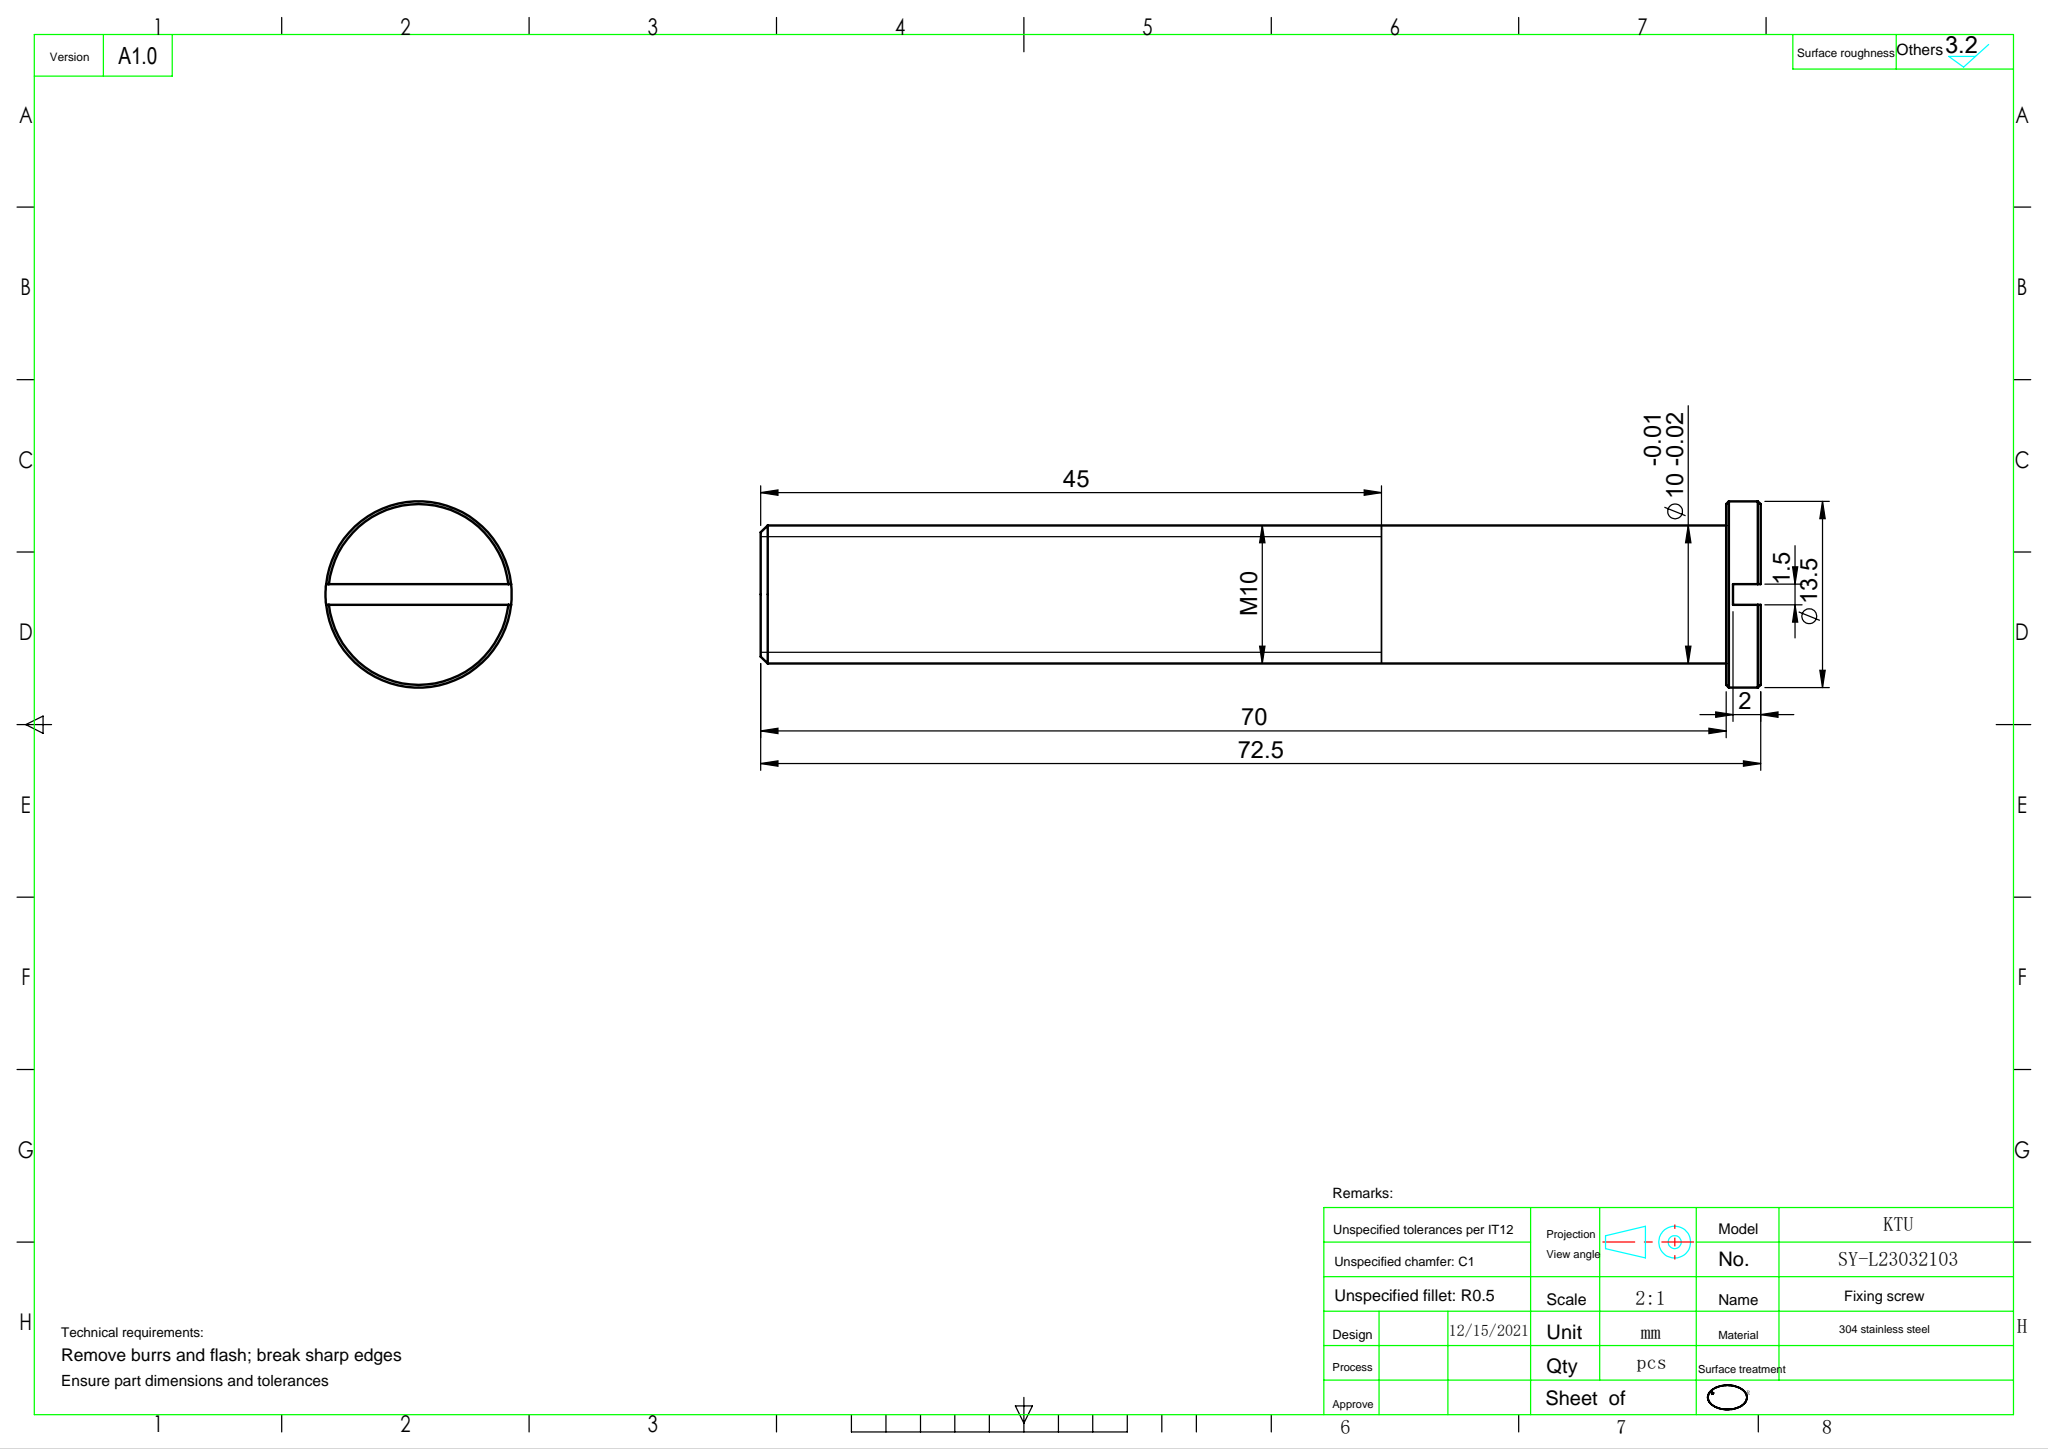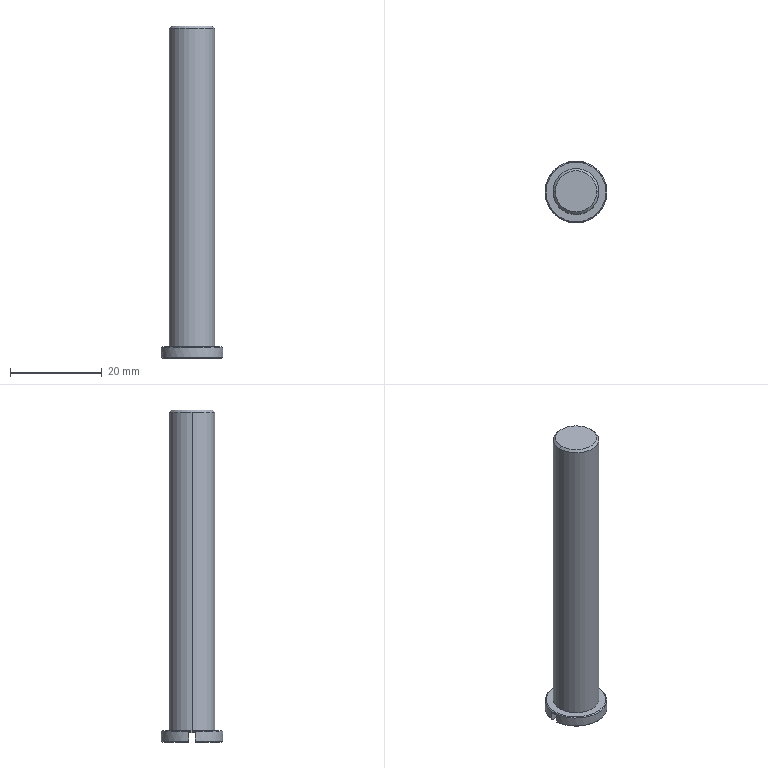Part | SolidWorks | features Chamfer 2, ICE 2, Extrusion 1 | 1 solid | 17 faces | box 13.5 x 13.5 x 72.5 mm | volume 5810 mm3 | plane 7 | cone 6 | cylinder 4 | commonest cylinder face diameters 10 x2 13.5 x2
STEP:
#1=CARTESIAN_POINT('',(6.55,0.,0.));
#2=VERTEX_POINT('',#1);
#3=CARTESIAN_POINT('',(-6.55,0.,0.));
#4=VERTEX_POINT('',#3);
#5=CARTESIAN_POINT('',(0.,0.,0.));
#6=DIRECTION('',(0.,0.,1.));
#7=DIRECTION('',(-1.,0.,0.));
#8=AXIS2_PLACEMENT_3D('',#5,#6,#7);
#9=CIRCLE('',#8,6.55);
#10=EDGE_CURVE('',#2,#4,#9,.T.);
#11=ORIENTED_EDGE('',*,*,#10,.F.);
#12=CARTESIAN_POINT('',(6.75,0.,-0.2));
#13=VERTEX_POINT('',#12);
#14=CARTESIAN_POINT('',(6.75,0.,-0.2));
#15=DIRECTION('',(0.7071,0.,-0.7071));
#16=VECTOR('',#15,1000.);
#17=LINE('',#14,#16);
#18=EDGE_CURVE('',#2,#13,#17,.T.);
#19=ORIENTED_EDGE('',*,*,#18,.T.);
#20=CARTESIAN_POINT('',(-6.75,0.,-0.2));
#21=VERTEX_POINT('',#20);
#22=CARTESIAN_POINT('',(0.,0.,-0.2));
#23=DIRECTION('',(0.,0.,-1.));
#24=DIRECTION('',(-1.,0.,0.));
#25=AXIS2_PLACEMENT_3D('',#22,#23,#24);
#26=CIRCLE('',#25,6.75);
#27=EDGE_CURVE('',#21,#13,#26,.T.);
#28=ORIENTED_EDGE('',*,*,#27,.F.);
#29=CARTESIAN_POINT('',(-6.75,0.,-0.2));
#30=DIRECTION('',(-0.7071,0.,-0.7071));
#31=VECTOR('',#30,1000.);
#32=LINE('',#29,#31);
#33=EDGE_CURVE('',#4,#21,#32,.T.);
#34=ORIENTED_EDGE('',*,*,#33,.F.);
#35=EDGE_LOOP('',(#11,#19,#28,#34));
#36=FACE_OUTER_BOUND('',#35,.T.);
#37=CARTESIAN_POINT('',(0.,0.,-0.2));
#38=DIRECTION('',(0.,0.,-1.));
#39=DIRECTION('',(-1.,0.,0.));
#40=AXIS2_PLACEMENT_3D('',#37,#38,#39);
#41=CONICAL_SURFACE('',#40,6.75,0.7854);
#42=ADVANCED_FACE('',(#36),#41,.T.);
#43=CARTESIAN_POINT('',(4.5,0.,70.));
#44=VERTEX_POINT('',#43);
#45=CARTESIAN_POINT('',(-4.5,0.,70.));
#46=VERTEX_POINT('',#45);
#47=CARTESIAN_POINT('',(0.,0.,70.));
#48=DIRECTION('',(0.,0.,1.));
#49=DIRECTION('',(1.,0.,0.));
#50=AXIS2_PLACEMENT_3D('',#47,#48,#49);
#51=CIRCLE('',#50,4.5);
#52=EDGE_CURVE('',#44,#46,#51,.T.);
#53=ORIENTED_EDGE('',*,*,#52,.F.);
#54=CARTESIAN_POINT('',(5.,0.,69.5));
#55=VERTEX_POINT('',#54);
#56=CARTESIAN_POINT('',(4.5,0.,70.));
#57=DIRECTION('',(0.7071,0.,-0.7071));
#58=VECTOR('',#57,1000.);
#59=LINE('',#56,#58);
#60=EDGE_CURVE('',#44,#55,#59,.T.);
#61=ORIENTED_EDGE('',*,*,#60,.T.);
#62=CARTESIAN_POINT('',(-5.,0.,69.5));
#63=VERTEX_POINT('',#62);
#64=CARTESIAN_POINT('',(0.,0.,69.5));
#65=DIRECTION('',(0.,0.,-1.));
#66=DIRECTION('',(1.,0.,0.));
#67=AXIS2_PLACEMENT_3D('',#64,#65,#66);
#68=CIRCLE('',#67,5.);
#69=EDGE_CURVE('',#63,#55,#68,.T.);
#70=ORIENTED_EDGE('',*,*,#69,.F.);
#71=CARTESIAN_POINT('',(-4.5,0.,70.));
#72=DIRECTION('',(-0.7071,0.,-0.7071));
#73=VECTOR('',#72,1000.);
#74=LINE('',#71,#73);
#75=EDGE_CURVE('',#46,#63,#74,.T.);
#76=ORIENTED_EDGE('',*,*,#75,.F.);
#77=EDGE_LOOP('',(#53,#61,#70,#76));
#78=FACE_OUTER_BOUND('',#77,.T.);
#79=CARTESIAN_POINT('',(0.,0.,70.));
#80=DIRECTION('',(0.,0.,-1.));
#81=DIRECTION('',(-1.,0.,0.));
#82=AXIS2_PLACEMENT_3D('',#79,#80,#81);
#83=CONICAL_SURFACE('',#82,4.5,0.7854);
#84=ADVANCED_FACE('',(#78),#83,.T.);
#85=CARTESIAN_POINT('',(-6.75,0.,-0.5));
#86=VERTEX_POINT('',#85);
#87=CARTESIAN_POINT('',(-6.708,0.75,-0.5));
#88=VERTEX_POINT('',#87);
#89=CARTESIAN_POINT('',(0.,0.,-0.5));
#90=DIRECTION('',(0.,0.,-1.));
#91=DIRECTION('',(-1.,0.,0.));
#92=AXIS2_PLACEMENT_3D('',#89,#90,#91);
#93=CIRCLE('',#92,6.75);
#94=EDGE_CURVE('',#86,#88,#93,.T.);
#95=ORIENTED_EDGE('',*,*,#94,.F.);
#96=CARTESIAN_POINT('',(-6.75,0.,-2.5));
#97=DIRECTION('',(0.,0.,1.));
#98=VECTOR('',#97,1000.);
#99=LINE('',#96,#98);
#100=EDGE_CURVE('',#86,#21,#99,.T.);
#101=ORIENTED_EDGE('',*,*,#100,.T.);
#102=ORIENTED_EDGE('',*,*,#27,.T.);
#103=CARTESIAN_POINT('',(6.75,0.,-0.5));
#104=VERTEX_POINT('',#103);
#105=CARTESIAN_POINT('',(6.75,0.,-2.5));
#106=DIRECTION('',(0.,0.,1.));
#107=VECTOR('',#106,1000.);
#108=LINE('',#105,#107);
#109=EDGE_CURVE('',#104,#13,#108,.T.);
#110=ORIENTED_EDGE('',*,*,#109,.F.);
#111=CARTESIAN_POINT('',(6.708,0.75,-0.5));
#112=VERTEX_POINT('',#111);
#113=CARTESIAN_POINT('',(0.,0.,-0.5));
#114=DIRECTION('',(0.,0.,-1.));
#115=DIRECTION('',(-1.,0.,0.));
#116=AXIS2_PLACEMENT_3D('',#113,#114,#115);
#117=CIRCLE('',#116,6.75);
#118=EDGE_CURVE('',#112,#104,#117,.T.);
#119=ORIENTED_EDGE('',*,*,#118,.F.);
#120=CARTESIAN_POINT('',(6.708,0.75,-2.3));
#121=VERTEX_POINT('',#120);
#122=CARTESIAN_POINT('',(6.708,0.75,-2.5));
#123=DIRECTION('',(0.,0.,-1.));
#124=VECTOR('',#123,1000.);
#125=LINE('',#122,#124);
#126=EDGE_CURVE('',#112,#121,#125,.T.);
#127=ORIENTED_EDGE('',*,*,#126,.T.);
#128=CARTESIAN_POINT('',(-6.708,0.75,-2.3));
#129=VERTEX_POINT('',#128);
#130=CARTESIAN_POINT('',(0.,0.,-2.3));
#131=DIRECTION('',(0.,0.,1.));
#132=DIRECTION('',(-1.,0.,0.));
#133=AXIS2_PLACEMENT_3D('',#130,#131,#132);
#134=CIRCLE('',#133,6.75);
#135=EDGE_CURVE('',#121,#129,#134,.T.);
#136=ORIENTED_EDGE('',*,*,#135,.T.);
#137=CARTESIAN_POINT('',(-6.708,0.75,-2.5));
#138=DIRECTION('',(0.,0.,1.));
#139=VECTOR('',#138,1000.);
#140=LINE('',#137,#139);
#141=EDGE_CURVE('',#129,#88,#140,.T.);
#142=ORIENTED_EDGE('',*,*,#141,.T.);
#143=EDGE_LOOP('',(#95,#101,#102,#110,#119,#127,#136,#142));
#144=FACE_OUTER_BOUND('',#143,.T.);
#145=CARTESIAN_POINT('',(0.,0.,-2.5));
#146=DIRECTION('',(0.,0.,1.));
#147=DIRECTION('',(1.,0.,0.));
#148=AXIS2_PLACEMENT_3D('',#145,#146,#147);
#149=CYLINDRICAL_SURFACE('',#148,6.75);
#150=ADVANCED_FACE('',(#144),#149,.T.);
#151=ORIENTED_EDGE('',*,*,#69,.T.);
#152=CARTESIAN_POINT('',(5.,0.,0.));
#153=VERTEX_POINT('',#152);
#154=CARTESIAN_POINT('',(5.,0.,70.));
#155=DIRECTION('',(0.,0.,-1.));
#156=VECTOR('',#155,1000.);
#157=LINE('',#154,#156);
#158=EDGE_CURVE('',#55,#153,#157,.T.);
#159=ORIENTED_EDGE('',*,*,#158,.T.);
#160=CARTESIAN_POINT('',(-5.,0.,0.));
#161=VERTEX_POINT('',#160);
#162=CARTESIAN_POINT('',(0.,0.,0.));
#163=DIRECTION('',(0.,0.,-1.));
#164=DIRECTION('',(-1.,0.,0.));
#165=AXIS2_PLACEMENT_3D('',#162,#163,#164);
#166=CIRCLE('',#165,5.);
#167=EDGE_CURVE('',#161,#153,#166,.T.);
#168=ORIENTED_EDGE('',*,*,#167,.F.);
#169=CARTESIAN_POINT('',(-5.,0.,70.));
#170=DIRECTION('',(0.,0.,-1.));
#171=VECTOR('',#170,1000.);
#172=LINE('',#169,#171);
#173=EDGE_CURVE('',#63,#161,#172,.T.);
#174=ORIENTED_EDGE('',*,*,#173,.F.);
#175=EDGE_LOOP('',(#151,#159,#168,#174));
#176=FACE_OUTER_BOUND('',#175,.T.);
#177=CARTESIAN_POINT('',(0.,0.,70.));
#178=DIRECTION('',(0.,0.,-1.));
#179=DIRECTION('',(-1.,0.,0.));
#180=AXIS2_PLACEMENT_3D('',#177,#178,#179);
#181=CYLINDRICAL_SURFACE('',#180,5.);
#182=ADVANCED_FACE('',(#176),#181,.T.);
#183=CARTESIAN_POINT('',(6.507,-0.75,-2.5));
#184=VERTEX_POINT('',#183);
#185=CARTESIAN_POINT('',(-6.507,-0.75,-2.5));
#186=VERTEX_POINT('',#185);
#187=CARTESIAN_POINT('',(7.5,-0.75,-2.5));
#188=DIRECTION('',(-1.,0.,0.));
#189=VECTOR('',#188,1000.);
#190=LINE('',#187,#189);
#191=EDGE_CURVE('',#184,#186,#190,.T.);
#192=ORIENTED_EDGE('',*,*,#191,.F.);
#193=CARTESIAN_POINT('',(0.,0.,-2.5));
#194=DIRECTION('',(0.,0.,-1.));
#195=DIRECTION('',(-1.,0.,0.));
#196=AXIS2_PLACEMENT_3D('',#193,#194,#195);
#197=CIRCLE('',#196,6.55);
#198=EDGE_CURVE('',#184,#186,#197,.T.);
#199=ORIENTED_EDGE('',*,*,#198,.T.);
#200=EDGE_LOOP('',(#192,#199));
#201=FACE_OUTER_BOUND('',#200,.T.);
#202=CARTESIAN_POINT('',(0.,0.,-2.5));
#203=DIRECTION('',(0.,0.,-1.));
#204=DIRECTION('',(-1.,0.,0.));
#205=AXIS2_PLACEMENT_3D('',#202,#203,#204);
#206=PLANE('',#205);
#207=ADVANCED_FACE('',(#201),#206,.T.);
#208=CARTESIAN_POINT('',(6.708,-0.75,-2.3));
#209=VERTEX_POINT('',#208);
#210=CARTESIAN_POINT('',(6.708,-0.75,-2.3));
#211=CARTESIAN_POINT('',(6.641,-0.75,-2.367));
#212=CARTESIAN_POINT('',(6.574,-0.75,-2.433));
#213=CARTESIAN_POINT('',(6.507,-0.75,-2.5));
#214=B_SPLINE_CURVE_WITH_KNOTS('',3,(#210,#211,#212,#213),.UNSPECIFIED.,.F.,.F.,(4,4),(0.01147,0.01176),.UNSPECIFIED.);
#215=EDGE_CURVE('',#209,#184,#214,.T.);
#216=ORIENTED_EDGE('',*,*,#215,.F.);
#217=CARTESIAN_POINT('',(-6.708,-0.75,-2.3));
#218=VERTEX_POINT('',#217);
#219=CARTESIAN_POINT('',(0.,0.,-2.3));
#220=DIRECTION('',(0.,0.,1.));
#221=DIRECTION('',(-1.,0.,0.));
#222=AXIS2_PLACEMENT_3D('',#219,#220,#221);
#223=CIRCLE('',#222,6.75);
#224=EDGE_CURVE('',#218,#209,#223,.T.);
#225=ORIENTED_EDGE('',*,*,#224,.F.);
#226=CARTESIAN_POINT('',(-6.507,-0.75,-2.5));
#227=CARTESIAN_POINT('',(-6.574,-0.75,-2.433));
#228=CARTESIAN_POINT('',(-6.641,-0.75,-2.367));
#229=CARTESIAN_POINT('',(-6.708,-0.75,-2.3));
#230=B_SPLINE_CURVE_WITH_KNOTS('',3,(#226,#227,#228,#229),.UNSPECIFIED.,.F.,.F.,(4,4),(0.02933,0.02961),.UNSPECIFIED.);
#231=EDGE_CURVE('',#186,#218,#230,.T.);
#232=ORIENTED_EDGE('',*,*,#231,.F.);
#233=ORIENTED_EDGE('',*,*,#198,.F.);
#234=EDGE_LOOP('',(#216,#225,#232,#233));
#235=FACE_OUTER_BOUND('',#234,.T.);
#236=CARTESIAN_POINT('',(0.,0.,-2.5));
#237=DIRECTION('',(0.,0.,1.));
#238=DIRECTION('',(1.,0.,0.));
#239=AXIS2_PLACEMENT_3D('',#236,#237,#238);
#240=CONICAL_SURFACE('',#239,6.55,0.7854);
#241=ADVANCED_FACE('',(#235),#240,.T.);
#242=ORIENTED_EDGE('',*,*,#158,.F.);
#243=CARTESIAN_POINT('',(0.,0.,69.5));
#244=DIRECTION('',(0.,0.,-1.));
#245=DIRECTION('',(1.,0.,0.));
#246=AXIS2_PLACEMENT_3D('',#243,#244,#245);
#247=CIRCLE('',#246,5.);
#248=EDGE_CURVE('',#55,#63,#247,.T.);
#249=ORIENTED_EDGE('',*,*,#248,.T.);
#250=ORIENTED_EDGE('',*,*,#173,.T.);
#251=CARTESIAN_POINT('',(0.,0.,0.));
#252=DIRECTION('',(0.,0.,-1.));
#253=DIRECTION('',(-1.,0.,0.));
#254=AXIS2_PLACEMENT_3D('',#251,#252,#253);
#255=CIRCLE('',#254,5.);
#256=EDGE_CURVE('',#153,#161,#255,.T.);
#257=ORIENTED_EDGE('',*,*,#256,.F.);
#258=EDGE_LOOP('',(#242,#249,#250,#257));
#259=FACE_OUTER_BOUND('',#258,.T.);
#260=CARTESIAN_POINT('',(0.,0.,70.));
#261=DIRECTION('',(0.,0.,-1.));
#262=DIRECTION('',(-1.,0.,0.));
#263=AXIS2_PLACEMENT_3D('',#260,#261,#262);
#264=CYLINDRICAL_SURFACE('',#263,5.);
#265=ADVANCED_FACE('',(#259),#264,.T.);
#266=CARTESIAN_POINT('',(0.,0.,70.));
#267=DIRECTION('',(0.,0.,1.));
#268=DIRECTION('',(1.,0.,0.));
#269=AXIS2_PLACEMENT_3D('',#266,#267,#268);
#270=CIRCLE('',#269,4.5);
#271=EDGE_CURVE('',#46,#44,#270,.T.);
#272=ORIENTED_EDGE('',*,*,#271,.T.);
#273=ORIENTED_EDGE('',*,*,#52,.T.);
#274=EDGE_LOOP('',(#272,#273));
#275=FACE_OUTER_BOUND('',#274,.T.);
#276=CARTESIAN_POINT('',(0.,0.,70.));
#277=DIRECTION('',(0.,0.,1.));
#278=DIRECTION('',(1.,0.,0.));
#279=AXIS2_PLACEMENT_3D('',#276,#277,#278);
#280=PLANE('',#279);
#281=ADVANCED_FACE('',(#275),#280,.T.);
#282=ORIENTED_EDGE('',*,*,#100,.F.);
#283=CARTESIAN_POINT('',(-6.708,-0.75,-0.5));
#284=VERTEX_POINT('',#283);
#285=CARTESIAN_POINT('',(0.,0.,-0.5));
#286=DIRECTION('',(0.,0.,-1.));
#287=DIRECTION('',(-1.,0.,0.));
#288=AXIS2_PLACEMENT_3D('',#285,#286,#287);
#289=CIRCLE('',#288,6.75);
#290=EDGE_CURVE('',#284,#86,#289,.T.);
#291=ORIENTED_EDGE('',*,*,#290,.F.);
#292=CARTESIAN_POINT('',(-6.708,-0.75,-2.5));
#293=DIRECTION('',(0.,0.,-1.));
#294=VECTOR('',#293,1000.);
#295=LINE('',#292,#294);
#296=EDGE_CURVE('',#284,#218,#295,.T.);
#297=ORIENTED_EDGE('',*,*,#296,.T.);
#298=ORIENTED_EDGE('',*,*,#224,.T.);
#299=CARTESIAN_POINT('',(6.708,-0.75,-0.5));
#300=VERTEX_POINT('',#299);
#301=CARTESIAN_POINT('',(6.708,-0.75,-2.5));
#302=DIRECTION('',(0.,0.,1.));
#303=VECTOR('',#302,1000.);
#304=LINE('',#301,#303);
#305=EDGE_CURVE('',#209,#300,#304,.T.);
#306=ORIENTED_EDGE('',*,*,#305,.T.);
#307=CARTESIAN_POINT('',(0.,0.,-0.5));
#308=DIRECTION('',(0.,0.,-1.));
#309=DIRECTION('',(-1.,0.,0.));
#310=AXIS2_PLACEMENT_3D('',#307,#308,#309);
#311=CIRCLE('',#310,6.75);
#312=EDGE_CURVE('',#104,#300,#311,.T.);
#313=ORIENTED_EDGE('',*,*,#312,.F.);
#314=ORIENTED_EDGE('',*,*,#109,.T.);
#315=CARTESIAN_POINT('',(0.,0.,-0.2));
#316=DIRECTION('',(0.,0.,-1.));
#317=DIRECTION('',(-1.,0.,0.));
#318=AXIS2_PLACEMENT_3D('',#315,#316,#317);
#319=CIRCLE('',#318,6.75);
#320=EDGE_CURVE('',#13,#21,#319,.T.);
#321=ORIENTED_EDGE('',*,*,#320,.T.);
#322=EDGE_LOOP('',(#282,#291,#297,#298,#306,#313,#314,#321));
#323=FACE_OUTER_BOUND('',#322,.T.);
#324=CARTESIAN_POINT('',(0.,0.,-2.5));
#325=DIRECTION('',(0.,0.,1.));
#326=DIRECTION('',(1.,0.,0.));
#327=AXIS2_PLACEMENT_3D('',#324,#325,#326);
#328=CYLINDRICAL_SURFACE('',#327,6.75);
#329=ADVANCED_FACE('',(#323),#328,.T.);
#330=CARTESIAN_POINT('',(-6.507,0.75,-2.5));
#331=VERTEX_POINT('',#330);
#332=CARTESIAN_POINT('',(6.507,0.75,-2.5));
#333=VERTEX_POINT('',#332);
#334=CARTESIAN_POINT('',(7.5,0.75,-2.5));
#335=DIRECTION('',(1.,0.,0.));
#336=VECTOR('',#335,1000.);
#337=LINE('',#334,#336);
#338=EDGE_CURVE('',#331,#333,#337,.T.);
#339=ORIENTED_EDGE('',*,*,#338,.F.);
#340=CARTESIAN_POINT('',(0.,0.,-2.5));
#341=DIRECTION('',(0.,0.,-1.));
#342=DIRECTION('',(-1.,0.,0.));
#343=AXIS2_PLACEMENT_3D('',#340,#341,#342);
#344=CIRCLE('',#343,6.55);
#345=EDGE_CURVE('',#331,#333,#344,.T.);
#346=ORIENTED_EDGE('',*,*,#345,.T.);
#347=EDGE_LOOP('',(#339,#346));
#348=FACE_OUTER_BOUND('',#347,.T.);
#349=CARTESIAN_POINT('',(0.,0.,-2.5));
#350=DIRECTION('',(0.,0.,-1.));
#351=DIRECTION('',(-1.,0.,0.));
#352=AXIS2_PLACEMENT_3D('',#349,#350,#351);
#353=PLANE('',#352);
#354=ADVANCED_FACE('',(#348),#353,.T.);
#355=CARTESIAN_POINT('',(0.,0.,0.));
#356=DIRECTION('',(0.,0.,1.));
#357=DIRECTION('',(-1.,0.,0.));
#358=AXIS2_PLACEMENT_3D('',#355,#356,#357);
#359=CIRCLE('',#358,6.55);
#360=EDGE_CURVE('',#4,#2,#359,.T.);
#361=ORIENTED_EDGE('',*,*,#360,.T.);
#362=ORIENTED_EDGE('',*,*,#10,.T.);
#363=EDGE_LOOP('',(#361,#362));
#364=FACE_OUTER_BOUND('',#363,.T.);
#365=ORIENTED_EDGE('',*,*,#167,.T.);
#366=ORIENTED_EDGE('',*,*,#256,.T.);
#367=EDGE_LOOP('',(#365,#366));
#368=FACE_BOUND('',#367,.T.);
#369=CARTESIAN_POINT('',(0.,0.,0.));
#370=DIRECTION('',(0.,0.,-1.));
#371=DIRECTION('',(-1.,0.,0.));
#372=AXIS2_PLACEMENT_3D('',#369,#370,#371);
#373=PLANE('',#372);
#374=ADVANCED_FACE('',(#364,#368),#373,.F.);
#375=ORIENTED_EDGE('',*,*,#60,.F.);
#376=ORIENTED_EDGE('',*,*,#271,.F.);
#377=ORIENTED_EDGE('',*,*,#75,.T.);
#378=ORIENTED_EDGE('',*,*,#248,.F.);
#379=EDGE_LOOP('',(#375,#376,#377,#378));
#380=FACE_OUTER_BOUND('',#379,.T.);
#381=CARTESIAN_POINT('',(0.,0.,70.));
#382=DIRECTION('',(0.,0.,-1.));
#383=DIRECTION('',(-1.,0.,0.));
#384=AXIS2_PLACEMENT_3D('',#381,#382,#383);
#385=CONICAL_SURFACE('',#384,4.5,0.7854);
#386=ADVANCED_FACE('',(#380),#385,.T.);
#387=CARTESIAN_POINT('',(-6.708,0.75,-2.3));
#388=CARTESIAN_POINT('',(-6.641,0.75,-2.367));
#389=CARTESIAN_POINT('',(-6.574,0.75,-2.433));
#390=CARTESIAN_POINT('',(-6.507,0.75,-2.5));
#391=B_SPLINE_CURVE_WITH_KNOTS('',3,(#387,#388,#389,#390),.UNSPECIFIED.,.F.,.F.,(4,4),(0.01147,0.01176),.UNSPECIFIED.);
#392=EDGE_CURVE('',#129,#331,#391,.T.);
#393=ORIENTED_EDGE('',*,*,#392,.F.);
#394=ORIENTED_EDGE('',*,*,#135,.F.);
#395=CARTESIAN_POINT('',(6.507,0.75,-2.5));
#396=CARTESIAN_POINT('',(6.574,0.75,-2.433));
#397=CARTESIAN_POINT('',(6.641,0.75,-2.367));
#398=CARTESIAN_POINT('',(6.708,0.75,-2.3));
#399=B_SPLINE_CURVE_WITH_KNOTS('',3,(#395,#396,#397,#398),.UNSPECIFIED.,.F.,.F.,(4,4),(0.02933,0.02961),.UNSPECIFIED.);
#400=EDGE_CURVE('',#333,#121,#399,.T.);
#401=ORIENTED_EDGE('',*,*,#400,.F.);
#402=ORIENTED_EDGE('',*,*,#345,.F.);
#403=EDGE_LOOP('',(#393,#394,#401,#402));
#404=FACE_OUTER_BOUND('',#403,.T.);
#405=CARTESIAN_POINT('',(0.,0.,-2.5));
#406=DIRECTION('',(0.,0.,1.));
#407=DIRECTION('',(1.,0.,0.));
#408=AXIS2_PLACEMENT_3D('',#405,#406,#407);
#409=CONICAL_SURFACE('',#408,6.55,0.7854);
#410=ADVANCED_FACE('',(#404),#409,.T.);
#411=ORIENTED_EDGE('',*,*,#18,.F.);
#412=ORIENTED_EDGE('',*,*,#360,.F.);
#413=ORIENTED_EDGE('',*,*,#33,.T.);
#414=ORIENTED_EDGE('',*,*,#320,.F.);
#415=EDGE_LOOP('',(#411,#412,#413,#414));
#416=FACE_OUTER_BOUND('',#415,.T.);
#417=CARTESIAN_POINT('',(0.,0.,-0.2));
#418=DIRECTION('',(0.,0.,-1.));
#419=DIRECTION('',(-1.,0.,0.));
#420=AXIS2_PLACEMENT_3D('',#417,#418,#419);
#421=CONICAL_SURFACE('',#420,6.75,0.7854);
#422=ADVANCED_FACE('',(#416),#421,.T.);
#423=ORIENTED_EDGE('',*,*,#118,.T.);
#424=ORIENTED_EDGE('',*,*,#312,.T.);
#425=CARTESIAN_POINT('',(7.5,-0.75,-0.5));
#426=DIRECTION('',(-1.,0.,0.));
#427=VECTOR('',#426,1000.);
#428=LINE('',#425,#427);
#429=EDGE_CURVE('',#300,#284,#428,.T.);
#430=ORIENTED_EDGE('',*,*,#429,.T.);
#431=ORIENTED_EDGE('',*,*,#290,.T.);
#432=ORIENTED_EDGE('',*,*,#94,.T.);
#433=CARTESIAN_POINT('',(7.5,0.75,-0.5));
#434=DIRECTION('',(1.,0.,0.));
#435=VECTOR('',#434,1000.);
#436=LINE('',#433,#435);
#437=EDGE_CURVE('',#88,#112,#436,.T.);
#438=ORIENTED_EDGE('',*,*,#437,.T.);
#439=EDGE_LOOP('',(#423,#424,#430,#431,#432,#438));
#440=FACE_OUTER_BOUND('',#439,.T.);
#441=CARTESIAN_POINT('',(0.,0.,-0.5));
#442=DIRECTION('',(0.,0.,-1.));
#443=DIRECTION('',(-1.,0.,0.));
#444=AXIS2_PLACEMENT_3D('',#441,#442,#443);
#445=PLANE('',#444);
#446=ADVANCED_FACE('',(#440),#445,.T.);
#447=ORIENTED_EDGE('',*,*,#215,.T.);
#448=ORIENTED_EDGE('',*,*,#191,.T.);
#449=ORIENTED_EDGE('',*,*,#231,.T.);
#450=ORIENTED_EDGE('',*,*,#296,.F.);
#451=ORIENTED_EDGE('',*,*,#429,.F.);
#452=ORIENTED_EDGE('',*,*,#305,.F.);
#453=EDGE_LOOP('',(#447,#448,#449,#450,#451,#452));
#454=FACE_OUTER_BOUND('',#453,.T.);
#455=CARTESIAN_POINT('',(7.5,-0.75,-0.5));
#456=DIRECTION('',(0.,-1.,0.));
#457=DIRECTION('',(0.,0.,-1.));
#458=AXIS2_PLACEMENT_3D('',#455,#456,#457);
#459=PLANE('',#458);
#460=ADVANCED_FACE('',(#454),#459,.F.);
#461=ORIENTED_EDGE('',*,*,#392,.T.);
#462=ORIENTED_EDGE('',*,*,#338,.T.);
#463=ORIENTED_EDGE('',*,*,#400,.T.);
#464=ORIENTED_EDGE('',*,*,#126,.F.);
#465=ORIENTED_EDGE('',*,*,#437,.F.);
#466=ORIENTED_EDGE('',*,*,#141,.F.);
#467=EDGE_LOOP('',(#461,#462,#463,#464,#465,#466));
#468=FACE_OUTER_BOUND('',#467,.T.);
#469=CARTESIAN_POINT('',(7.5,0.75,-0.5));
#470=DIRECTION('',(0.,1.,0.));
#471=DIRECTION('',(0.,0.,1.));
#472=AXIS2_PLACEMENT_3D('',#469,#470,#471);
#473=PLANE('',#472);
#474=ADVANCED_FACE('',(#468),#473,.F.);
#475=CLOSED_SHELL('',(#42,#84,#150,#182,#207,#241,#265,#281,#329,#354,#374,#386,#410,#422,#446,#460,#474));
#476=MANIFOLD_SOLID_BREP('',#475);
#477=CARTESIAN_POINT('',(0.,0.,0.));
#478=DIRECTION('',(0.,0.,1.));
#479=DIRECTION('',(1.,0.,0.));
#480=AXIS2_PLACEMENT_3D('',#477,#478,#479);
#481=(LENGTH_UNIT()NAMED_UNIT(*)SI_UNIT(.MILLI.,.METRE.));
#482=UNCERTAINTY_MEASURE_WITH_UNIT(LENGTH_MEASURE(0.00001),#481,'','');
#483=(NAMED_UNIT(*)PLANE_ANGLE_UNIT()SI_UNIT($,.RADIAN.));
#484=(NAMED_UNIT(*)SI_UNIT($,.STERADIAN.)SOLID_ANGLE_UNIT());
#485=(GEOMETRIC_REPRESENTATION_CONTEXT(3)GLOBAL_UNCERTAINTY_ASSIGNED_CONTEXT((#482))GLOBAL_UNIT_ASSIGNED_CONTEXT((#481,#483,#484))REPRESENTATION_CONTEXT('',''));
#486=ADVANCED_BREP_SHAPE_REPRESENTATION('',(#476,#480),#485);